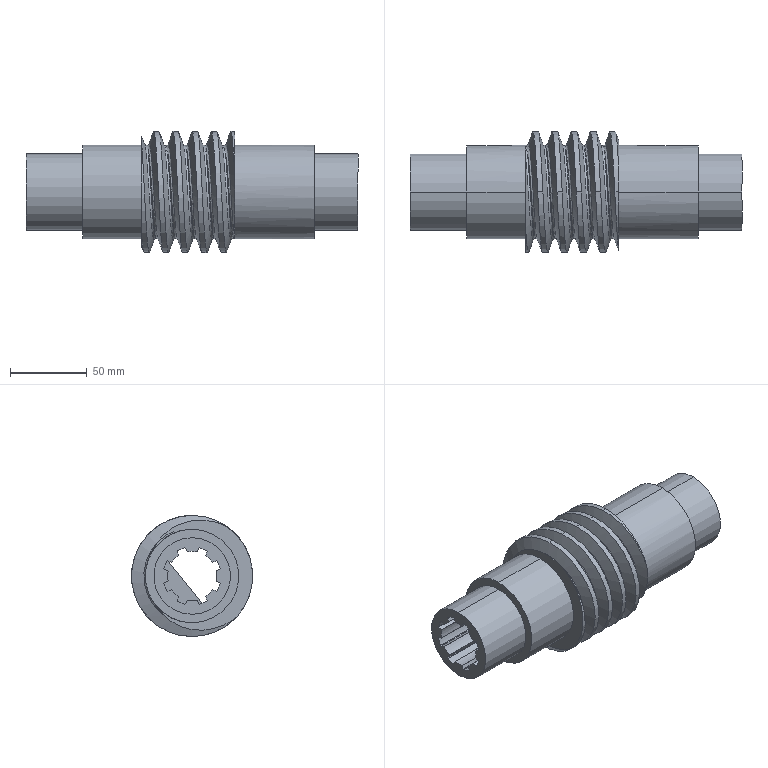Part | SolidWorks | features BaseBody 1 | 1 solid | 99 faces | box 216.6 x 79 x 79 mm | volume 426843 mm3 | cylinder 56 | plane 38 | spline 5 | commonest cylinder face diameters 0.2 x20 79 x11 32 x9 38 x8 50 x4 61 x4